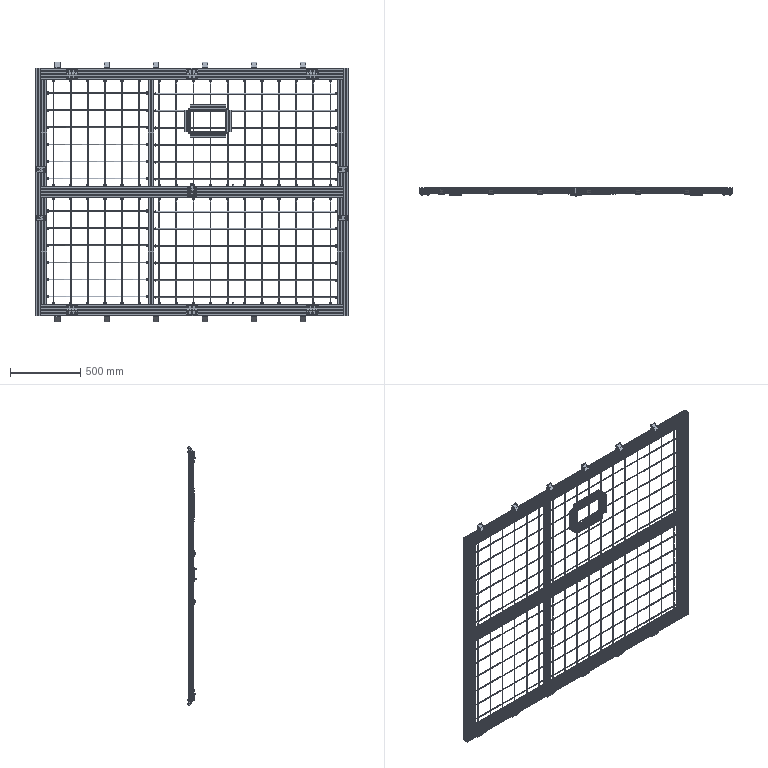Part | 306 solids | 12473 faces | volume 13535631 mm3 | plane 7331 | cylinder 3950 | cone 1104 | spline 88 | commonest cylinder face diameters 16.3 x580 10 x466 0.6 x432 2 x412 4.5 x232 4.6 x232